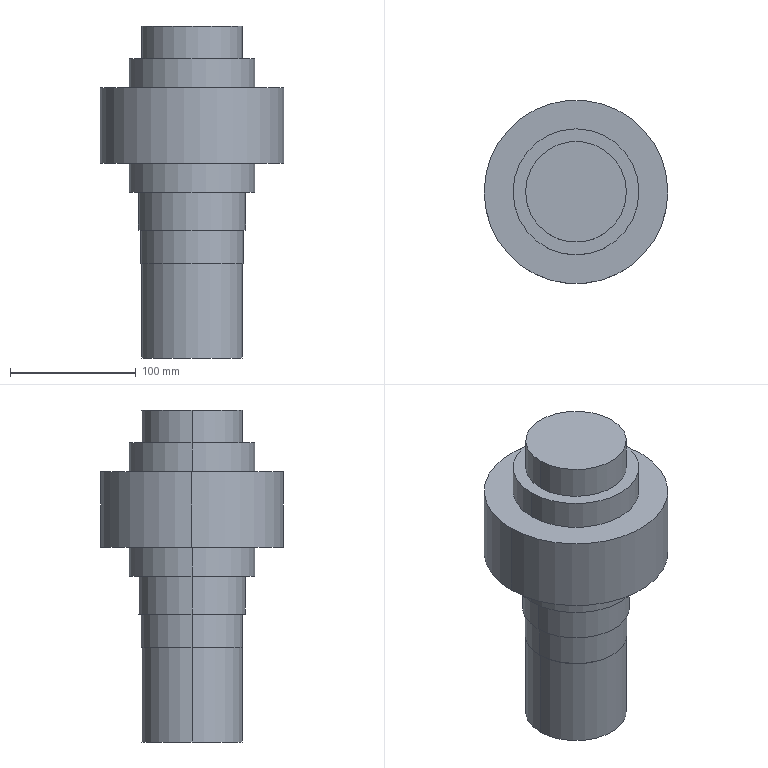Part | SolidWorks | features ICE 6, Extrusion 1 | 1 solid | 22 faces | box 145.723 x 145.723 x 263.5 mm | volume 2176439 mm3 | cylinder 14 | plane 8 | commonest cylinder face diameters 80 x4 100 x4 81 x2 85 x2 145.723 x2
STEP:
#1=CARTESIAN_POINT('',(-40.,0.,-237.5));
#2=VERTEX_POINT('',#1);
#3=CARTESIAN_POINT('',(40.,0.,-237.5));
#4=VERTEX_POINT('',#3);
#5=CARTESIAN_POINT('',(0.,0.,-237.5));
#6=DIRECTION('',(0.,0.,-1.));
#7=DIRECTION('',(-1.,0.,0.));
#8=AXIS2_PLACEMENT_3D('',#5,#6,#7);
#9=CIRCLE('',#8,40.);
#10=EDGE_CURVE('',#2,#4,#9,.T.);
#11=ORIENTED_EDGE('',*,*,#10,.F.);
#12=CARTESIAN_POINT('',(-40.,0.,-162.5));
#13=VERTEX_POINT('',#12);
#14=CARTESIAN_POINT('',(-40.,0.,-237.5));
#15=DIRECTION('',(0.,0.,1.));
#16=VECTOR('',#15,1000.);
#17=LINE('',#14,#16);
#18=EDGE_CURVE('',#2,#13,#17,.T.);
#19=ORIENTED_EDGE('',*,*,#18,.T.);
#20=CARTESIAN_POINT('',(40.,0.,-162.5));
#21=VERTEX_POINT('',#20);
#22=CARTESIAN_POINT('',(0.,0.,-162.5));
#23=DIRECTION('',(0.,0.,-1.));
#24=DIRECTION('',(-1.,0.,0.));
#25=AXIS2_PLACEMENT_3D('',#22,#23,#24);
#26=CIRCLE('',#25,40.);
#27=EDGE_CURVE('',#13,#21,#26,.T.);
#28=ORIENTED_EDGE('',*,*,#27,.T.);
#29=CARTESIAN_POINT('',(40.,0.,-237.5));
#30=DIRECTION('',(0.,0.,1.));
#31=VECTOR('',#30,1000.);
#32=LINE('',#29,#31);
#33=EDGE_CURVE('',#4,#21,#32,.T.);
#34=ORIENTED_EDGE('',*,*,#33,.F.);
#35=EDGE_LOOP('',(#11,#19,#28,#34));
#36=FACE_OUTER_BOUND('',#35,.T.);
#37=CARTESIAN_POINT('',(0.,0.,-237.5));
#38=DIRECTION('',(0.,0.,1.));
#39=DIRECTION('',(1.,0.,0.));
#40=AXIS2_PLACEMENT_3D('',#37,#38,#39);
#41=CYLINDRICAL_SURFACE('',#40,40.);
#42=ADVANCED_FACE('',(#36),#41,.T.);
#43=CARTESIAN_POINT('',(-40.5,0.,-162.5));
#44=VERTEX_POINT('',#43);
#45=CARTESIAN_POINT('',(40.5,0.,-162.5));
#46=VERTEX_POINT('',#45);
#47=CARTESIAN_POINT('',(0.,0.,-162.5));
#48=DIRECTION('',(0.,0.,-1.));
#49=DIRECTION('',(-1.,0.,0.));
#50=AXIS2_PLACEMENT_3D('',#47,#48,#49);
#51=CIRCLE('',#50,40.5);
#52=EDGE_CURVE('',#44,#46,#51,.T.);
#53=ORIENTED_EDGE('',*,*,#52,.F.);
#54=CARTESIAN_POINT('',(-40.5,0.,-136.));
#55=VERTEX_POINT('',#54);
#56=CARTESIAN_POINT('',(-40.5,0.,-162.5));
#57=DIRECTION('',(0.,0.,1.));
#58=VECTOR('',#57,1000.);
#59=LINE('',#56,#58);
#60=EDGE_CURVE('',#44,#55,#59,.T.);
#61=ORIENTED_EDGE('',*,*,#60,.T.);
#62=CARTESIAN_POINT('',(40.5,0.,-136.));
#63=VERTEX_POINT('',#62);
#64=CARTESIAN_POINT('',(0.,0.,-136.));
#65=DIRECTION('',(0.,0.,-1.));
#66=DIRECTION('',(-1.,0.,0.));
#67=AXIS2_PLACEMENT_3D('',#64,#65,#66);
#68=CIRCLE('',#67,40.5);
#69=EDGE_CURVE('',#55,#63,#68,.T.);
#70=ORIENTED_EDGE('',*,*,#69,.T.);
#71=CARTESIAN_POINT('',(40.5,0.,-162.5));
#72=DIRECTION('',(0.,0.,1.));
#73=VECTOR('',#72,1000.);
#74=LINE('',#71,#73);
#75=EDGE_CURVE('',#46,#63,#74,.T.);
#76=ORIENTED_EDGE('',*,*,#75,.F.);
#77=EDGE_LOOP('',(#53,#61,#70,#76));
#78=FACE_OUTER_BOUND('',#77,.T.);
#79=CARTESIAN_POINT('',(0.,0.,-162.5));
#80=DIRECTION('',(0.,0.,1.));
#81=DIRECTION('',(1.,0.,0.));
#82=AXIS2_PLACEMENT_3D('',#79,#80,#81);
#83=CYLINDRICAL_SURFACE('',#82,40.5);
#84=ADVANCED_FACE('',(#78),#83,.T.);
#85=CARTESIAN_POINT('',(-42.5,0.,-136.));
#86=VERTEX_POINT('',#85);
#87=CARTESIAN_POINT('',(42.5,0.,-136.));
#88=VERTEX_POINT('',#87);
#89=CARTESIAN_POINT('',(0.,0.,-136.));
#90=DIRECTION('',(0.,0.,-1.));
#91=DIRECTION('',(-1.,0.,0.));
#92=AXIS2_PLACEMENT_3D('',#89,#90,#91);
#93=CIRCLE('',#92,42.5);
#94=EDGE_CURVE('',#86,#88,#93,.T.);
#95=ORIENTED_EDGE('',*,*,#94,.F.);
#96=CARTESIAN_POINT('',(-42.5,0.,-106.));
#97=VERTEX_POINT('',#96);
#98=CARTESIAN_POINT('',(-42.5,0.,-136.));
#99=DIRECTION('',(0.,0.,1.));
#100=VECTOR('',#99,1000.);
#101=LINE('',#98,#100);
#102=EDGE_CURVE('',#86,#97,#101,.T.);
#103=ORIENTED_EDGE('',*,*,#102,.T.);
#104=CARTESIAN_POINT('',(42.5,0.,-106.));
#105=VERTEX_POINT('',#104);
#106=CARTESIAN_POINT('',(0.,0.,-106.));
#107=DIRECTION('',(0.,0.,-1.));
#108=DIRECTION('',(-1.,0.,0.));
#109=AXIS2_PLACEMENT_3D('',#106,#107,#108);
#110=CIRCLE('',#109,42.5);
#111=EDGE_CURVE('',#97,#105,#110,.T.);
#112=ORIENTED_EDGE('',*,*,#111,.T.);
#113=CARTESIAN_POINT('',(42.5,0.,-136.));
#114=DIRECTION('',(0.,0.,1.));
#115=VECTOR('',#114,1000.);
#116=LINE('',#113,#115);
#117=EDGE_CURVE('',#88,#105,#116,.T.);
#118=ORIENTED_EDGE('',*,*,#117,.F.);
#119=EDGE_LOOP('',(#95,#103,#112,#118));
#120=FACE_OUTER_BOUND('',#119,.T.);
#121=CARTESIAN_POINT('',(0.,0.,-136.));
#122=DIRECTION('',(0.,0.,1.));
#123=DIRECTION('',(1.,0.,0.));
#124=AXIS2_PLACEMENT_3D('',#121,#122,#123);
#125=CYLINDRICAL_SURFACE('',#124,42.5);
#126=ADVANCED_FACE('',(#120),#125,.T.);
#127=CARTESIAN_POINT('',(-50.,0.,-106.));
#128=VERTEX_POINT('',#127);
#129=CARTESIAN_POINT('',(50.,0.,-106.));
#130=VERTEX_POINT('',#129);
#131=CARTESIAN_POINT('',(0.,0.,-106.));
#132=DIRECTION('',(0.,0.,-1.));
#133=DIRECTION('',(-1.,0.,0.));
#134=AXIS2_PLACEMENT_3D('',#131,#132,#133);
#135=CIRCLE('',#134,50.);
#136=EDGE_CURVE('',#128,#130,#135,.T.);
#137=ORIENTED_EDGE('',*,*,#136,.F.);
#138=CARTESIAN_POINT('',(-50.,0.,-83.));
#139=VERTEX_POINT('',#138);
#140=CARTESIAN_POINT('',(-50.,0.,-106.));
#141=DIRECTION('',(0.,0.,1.));
#142=VECTOR('',#141,1000.);
#143=LINE('',#140,#142);
#144=EDGE_CURVE('',#128,#139,#143,.T.);
#145=ORIENTED_EDGE('',*,*,#144,.T.);
#146=CARTESIAN_POINT('',(50.,0.,-83.));
#147=VERTEX_POINT('',#146);
#148=CARTESIAN_POINT('',(0.,0.,-83.));
#149=DIRECTION('',(0.,0.,-1.));
#150=DIRECTION('',(-1.,0.,0.));
#151=AXIS2_PLACEMENT_3D('',#148,#149,#150);
#152=CIRCLE('',#151,50.);
#153=EDGE_CURVE('',#139,#147,#152,.T.);
#154=ORIENTED_EDGE('',*,*,#153,.T.);
#155=CARTESIAN_POINT('',(50.,0.,-106.));
#156=DIRECTION('',(0.,0.,1.));
#157=VECTOR('',#156,1000.);
#158=LINE('',#155,#157);
#159=EDGE_CURVE('',#130,#147,#158,.T.);
#160=ORIENTED_EDGE('',*,*,#159,.F.);
#161=EDGE_LOOP('',(#137,#145,#154,#160));
#162=FACE_OUTER_BOUND('',#161,.T.);
#163=CARTESIAN_POINT('',(0.,0.,-106.));
#164=DIRECTION('',(0.,0.,1.));
#165=DIRECTION('',(1.,0.,0.));
#166=AXIS2_PLACEMENT_3D('',#163,#164,#165);
#167=CYLINDRICAL_SURFACE('',#166,50.);
#168=ADVANCED_FACE('',(#162),#167,.T.);
#169=CARTESIAN_POINT('',(-72.862,0.,-83.));
#170=VERTEX_POINT('',#169);
#171=CARTESIAN_POINT('',(72.862,0.,-83.));
#172=VERTEX_POINT('',#171);
#173=CARTESIAN_POINT('',(0.,0.,-83.));
#174=DIRECTION('',(0.,0.,-1.));
#175=DIRECTION('',(-1.,0.,0.));
#176=AXIS2_PLACEMENT_3D('',#173,#174,#175);
#177=CIRCLE('',#176,72.862);
#178=EDGE_CURVE('',#170,#172,#177,.T.);
#179=ORIENTED_EDGE('',*,*,#178,.F.);
#180=CARTESIAN_POINT('',(-72.862,0.,-23.));
#181=VERTEX_POINT('',#180);
#182=CARTESIAN_POINT('',(-72.862,0.,-83.));
#183=DIRECTION('',(0.,0.,1.));
#184=VECTOR('',#183,1000.);
#185=LINE('',#182,#184);
#186=EDGE_CURVE('',#170,#181,#185,.T.);
#187=ORIENTED_EDGE('',*,*,#186,.T.);
#188=CARTESIAN_POINT('',(72.862,0.,-23.));
#189=VERTEX_POINT('',#188);
#190=CARTESIAN_POINT('',(0.,0.,-23.));
#191=DIRECTION('',(0.,0.,-1.));
#192=DIRECTION('',(-1.,0.,0.));
#193=AXIS2_PLACEMENT_3D('',#190,#191,#192);
#194=CIRCLE('',#193,72.862);
#195=EDGE_CURVE('',#181,#189,#194,.T.);
#196=ORIENTED_EDGE('',*,*,#195,.T.);
#197=CARTESIAN_POINT('',(72.862,0.,-83.));
#198=DIRECTION('',(0.,0.,1.));
#199=VECTOR('',#198,1000.);
#200=LINE('',#197,#199);
#201=EDGE_CURVE('',#172,#189,#200,.T.);
#202=ORIENTED_EDGE('',*,*,#201,.F.);
#203=EDGE_LOOP('',(#179,#187,#196,#202));
#204=FACE_OUTER_BOUND('',#203,.T.);
#205=CARTESIAN_POINT('',(0.,0.,-83.));
#206=DIRECTION('',(0.,0.,1.));
#207=DIRECTION('',(1.,0.,0.));
#208=AXIS2_PLACEMENT_3D('',#205,#206,#207);
#209=CYLINDRICAL_SURFACE('',#208,72.862);
#210=ADVANCED_FACE('',(#204),#209,.T.);
#211=CARTESIAN_POINT('',(-50.,0.,-23.));
#212=VERTEX_POINT('',#211);
#213=CARTESIAN_POINT('',(50.,0.,-23.));
#214=VERTEX_POINT('',#213);
#215=CARTESIAN_POINT('',(0.,0.,-23.));
#216=DIRECTION('',(0.,0.,-1.));
#217=DIRECTION('',(-1.,0.,0.));
#218=AXIS2_PLACEMENT_3D('',#215,#216,#217);
#219=CIRCLE('',#218,50.);
#220=EDGE_CURVE('',#212,#214,#219,.T.);
#221=ORIENTED_EDGE('',*,*,#220,.F.);
#222=CARTESIAN_POINT('',(-50.,0.,0.));
#223=VERTEX_POINT('',#222);
#224=CARTESIAN_POINT('',(-50.,0.,-23.));
#225=DIRECTION('',(0.,0.,1.));
#226=VECTOR('',#225,1000.);
#227=LINE('',#224,#226);
#228=EDGE_CURVE('',#212,#223,#227,.T.);
#229=ORIENTED_EDGE('',*,*,#228,.T.);
#230=CARTESIAN_POINT('',(50.,0.,0.));
#231=VERTEX_POINT('',#230);
#232=CARTESIAN_POINT('',(0.,0.,0.));
#233=DIRECTION('',(0.,0.,-1.));
#234=DIRECTION('',(-1.,0.,0.));
#235=AXIS2_PLACEMENT_3D('',#232,#233,#234);
#236=CIRCLE('',#235,50.);
#237=EDGE_CURVE('',#223,#231,#236,.T.);
#238=ORIENTED_EDGE('',*,*,#237,.T.);
#239=CARTESIAN_POINT('',(50.,0.,-23.));
#240=DIRECTION('',(0.,0.,1.));
#241=VECTOR('',#240,1000.);
#242=LINE('',#239,#241);
#243=EDGE_CURVE('',#214,#231,#242,.T.);
#244=ORIENTED_EDGE('',*,*,#243,.F.);
#245=EDGE_LOOP('',(#221,#229,#238,#244));
#246=FACE_OUTER_BOUND('',#245,.T.);
#247=CARTESIAN_POINT('',(0.,0.,-23.));
#248=DIRECTION('',(0.,0.,1.));
#249=DIRECTION('',(1.,0.,0.));
#250=AXIS2_PLACEMENT_3D('',#247,#248,#249);
#251=CYLINDRICAL_SURFACE('',#250,50.);
#252=ADVANCED_FACE('',(#246),#251,.T.);
#253=CARTESIAN_POINT('',(40.,0.,26.));
#254=VERTEX_POINT('',#253);
#255=CARTESIAN_POINT('',(-40.,0.,26.));
#256=VERTEX_POINT('',#255);
#257=CARTESIAN_POINT('',(0.,0.,26.));
#258=DIRECTION('',(0.,0.,1.));
#259=DIRECTION('',(1.,0.,0.));
#260=AXIS2_PLACEMENT_3D('',#257,#258,#259);
#261=CIRCLE('',#260,40.);
#262=EDGE_CURVE('',#254,#256,#261,.T.);
#263=ORIENTED_EDGE('',*,*,#262,.F.);
#264=CARTESIAN_POINT('',(40.,0.,0.));
#265=VERTEX_POINT('',#264);
#266=CARTESIAN_POINT('',(40.,0.,26.));
#267=DIRECTION('',(0.,0.,-1.));
#268=VECTOR('',#267,1000.);
#269=LINE('',#266,#268);
#270=EDGE_CURVE('',#254,#265,#269,.T.);
#271=ORIENTED_EDGE('',*,*,#270,.T.);
#272=CARTESIAN_POINT('',(-40.,0.,0.));
#273=VERTEX_POINT('',#272);
#274=CARTESIAN_POINT('',(0.,0.,0.));
#275=DIRECTION('',(0.,0.,-1.));
#276=DIRECTION('',(-1.,0.,0.));
#277=AXIS2_PLACEMENT_3D('',#274,#275,#276);
#278=CIRCLE('',#277,40.);
#279=EDGE_CURVE('',#273,#265,#278,.T.);
#280=ORIENTED_EDGE('',*,*,#279,.F.);
#281=CARTESIAN_POINT('',(-40.,0.,26.));
#282=DIRECTION('',(0.,0.,-1.));
#283=VECTOR('',#282,1000.);
#284=LINE('',#281,#283);
#285=EDGE_CURVE('',#256,#273,#284,.T.);
#286=ORIENTED_EDGE('',*,*,#285,.F.);
#287=EDGE_LOOP('',(#263,#271,#280,#286));
#288=FACE_OUTER_BOUND('',#287,.T.);
#289=CARTESIAN_POINT('',(0.,0.,26.));
#290=DIRECTION('',(0.,0.,-1.));
#291=DIRECTION('',(-1.,0.,0.));
#292=AXIS2_PLACEMENT_3D('',#289,#290,#291);
#293=CYLINDRICAL_SURFACE('',#292,40.);
#294=ADVANCED_FACE('',(#288),#293,.T.);
#295=CARTESIAN_POINT('',(0.,0.,-162.5));
#296=DIRECTION('',(0.,0.,-1.));
#297=DIRECTION('',(-1.,0.,0.));
#298=AXIS2_PLACEMENT_3D('',#295,#296,#297);
#299=CIRCLE('',#298,40.5);
#300=EDGE_CURVE('',#46,#44,#299,.T.);
#301=ORIENTED_EDGE('',*,*,#300,.T.);
#302=ORIENTED_EDGE('',*,*,#52,.T.);
#303=EDGE_LOOP('',(#301,#302));
#304=FACE_OUTER_BOUND('',#303,.T.);
#305=CARTESIAN_POINT('',(0.,0.,-162.5));
#306=DIRECTION('',(0.,0.,-1.));
#307=DIRECTION('',(-1.,0.,0.));
#308=AXIS2_PLACEMENT_3D('',#305,#306,#307);
#309=CIRCLE('',#308,40.);
#310=EDGE_CURVE('',#21,#13,#309,.T.);
#311=ORIENTED_EDGE('',*,*,#310,.F.);
#312=ORIENTED_EDGE('',*,*,#27,.F.);
#313=EDGE_LOOP('',(#311,#312));
#314=FACE_BOUND('',#313,.T.);
#315=CARTESIAN_POINT('',(0.,0.,-162.5));
#316=DIRECTION('',(0.,0.,-1.));
#317=DIRECTION('',(-1.,0.,0.));
#318=AXIS2_PLACEMENT_3D('',#315,#316,#317);
#319=PLANE('',#318);
#320=ADVANCED_FACE('',(#304,#314),#319,.T.);
#321=CARTESIAN_POINT('',(0.,0.,-136.));
#322=DIRECTION('',(0.,0.,-1.));
#323=DIRECTION('',(-1.,0.,0.));
#324=AXIS2_PLACEMENT_3D('',#321,#322,#323);
#325=CIRCLE('',#324,42.5);
#326=EDGE_CURVE('',#88,#86,#325,.T.);
#327=ORIENTED_EDGE('',*,*,#326,.T.);
#328=ORIENTED_EDGE('',*,*,#94,.T.);
#329=EDGE_LOOP('',(#327,#328));
#330=FACE_OUTER_BOUND('',#329,.T.);
#331=CARTESIAN_POINT('',(0.,0.,-136.));
#332=DIRECTION('',(0.,0.,-1.));
#333=DIRECTION('',(-1.,0.,0.));
#334=AXIS2_PLACEMENT_3D('',#331,#332,#333);
#335=CIRCLE('',#334,40.5);
#336=EDGE_CURVE('',#63,#55,#335,.T.);
#337=ORIENTED_EDGE('',*,*,#336,.F.);
#338=ORIENTED_EDGE('',*,*,#69,.F.);
#339=EDGE_LOOP('',(#337,#338));
#340=FACE_BOUND('',#339,.T.);
#341=CARTESIAN_POINT('',(0.,0.,-136.));
#342=DIRECTION('',(0.,0.,-1.));
#343=DIRECTION('',(-1.,0.,0.));
#344=AXIS2_PLACEMENT_3D('',#341,#342,#343);
#345=PLANE('',#344);
#346=ADVANCED_FACE('',(#330,#340),#345,.T.);
#347=CARTESIAN_POINT('',(0.,0.,-106.));
#348=DIRECTION('',(0.,0.,-1.));
#349=DIRECTION('',(-1.,0.,0.));
#350=AXIS2_PLACEMENT_3D('',#347,#348,#349);
#351=CIRCLE('',#350,50.);
#352=EDGE_CURVE('',#130,#128,#351,.T.);
#353=ORIENTED_EDGE('',*,*,#352,.T.);
#354=ORIENTED_EDGE('',*,*,#136,.T.);
#355=EDGE_LOOP('',(#353,#354));
#356=FACE_OUTER_BOUND('',#355,.T.);
#357=CARTESIAN_POINT('',(0.,0.,-106.));
#358=DIRECTION('',(0.,0.,-1.));
#359=DIRECTION('',(-1.,0.,0.));
#360=AXIS2_PLACEMENT_3D('',#357,#358,#359);
#361=CIRCLE('',#360,42.5);
#362=EDGE_CURVE('',#105,#97,#361,.T.);
#363=ORIENTED_EDGE('',*,*,#362,.F.);
#364=ORIENTED_EDGE('',*,*,#111,.F.);
#365=EDGE_LOOP('',(#363,#364));
#366=FACE_BOUND('',#365,.T.);
#367=CARTESIAN_POINT('',(0.,0.,-106.));
#368=DIRECTION('',(0.,0.,-1.));
#369=DIRECTION('',(-1.,0.,0.));
#370=AXIS2_PLACEMENT_3D('',#367,#368,#369);
#371=PLANE('',#370);
#372=ADVANCED_FACE('',(#356,#366),#371,.T.);
#373=CARTESIAN_POINT('',(0.,0.,-83.));
#374=DIRECTION('',(0.,0.,-1.));
#375=DIRECTION('',(-1.,0.,0.));
#376=AXIS2_PLACEMENT_3D('',#373,#374,#375);
#377=CIRCLE('',#376,72.862);
#378=EDGE_CURVE('',#172,#170,#377,.T.);
#379=ORIENTED_EDGE('',*,*,#378,.T.);
#380=ORIENTED_EDGE('',*,*,#178,.T.);
#381=EDGE_LOOP('',(#379,#380));
#382=FACE_OUTER_BOUND('',#381,.T.);
#383=CARTESIAN_POINT('',(0.,0.,-83.));
#384=DIRECTION('',(0.,0.,-1.));
#385=DIRECTION('',(-1.,0.,0.));
#386=AXIS2_PLACEMENT_3D('',#383,#384,#385);
#387=CIRCLE('',#386,50.);
#388=EDGE_CURVE('',#147,#139,#387,.T.);
#389=ORIENTED_EDGE('',*,*,#388,.F.);
#390=ORIENTED_EDGE('',*,*,#153,.F.);
#391=EDGE_LOOP('',(#389,#390));
#392=FACE_BOUND('',#391,.T.);
#393=CARTESIAN_POINT('',(0.,0.,-83.));
#394=DIRECTION('',(0.,0.,-1.));
#395=DIRECTION('',(-1.,0.,0.));
#396=AXIS2_PLACEMENT_3D('',#393,#394,#395);
#397=PLANE('',#396);
#398=ADVANCED_FACE('',(#382,#392),#397,.T.);
#399=ORIENTED_EDGE('',*,*,#270,.F.);
#400=CARTESIAN_POINT('',(0.,0.,26.));
#401=DIRECTION('',(0.,0.,1.));
#402=DIRECTION('',(1.,0.,0.));
#403=AXIS2_PLACEMENT_3D('',#400,#401,#402);
#404=CIRCLE('',#403,40.);
#405=EDGE_CURVE('',#256,#254,#404,.T.);
#406=ORIENTED_EDGE('',*,*,#405,.F.);
#407=ORIENTED_EDGE('',*,*,#285,.T.);
#408=CARTESIAN_POINT('',(0.,0.,0.));
#409=DIRECTION('',(0.,0.,-1.));
#410=DIRECTION('',(-1.,0.,0.));
#411=AXIS2_PLACEMENT_3D('',#408,#409,#410);
#412=CIRCLE('',#411,40.);
#413=EDGE_CURVE('',#265,#273,#412,.T.);
#414=ORIENTED_EDGE('',*,*,#413,.F.);
#415=EDGE_LOOP('',(#399,#406,#407,#414));
#416=FACE_OUTER_BOUND('',#415,.T.);
#417=CARTESIAN_POINT('',(0.,0.,26.));
#418=DIRECTION('',(0.,0.,-1.));
#419=DIRECTION('',(-1.,0.,0.));
#420=AXIS2_PLACEMENT_3D('',#417,#418,#419);
#421=CYLINDRICAL_SURFACE('',#420,40.);
#422=ADVANCED_FACE('',(#416),#421,.T.);
#423=ORIENTED_EDGE('',*,*,#405,.T.);
#424=ORIENTED_EDGE('',*,*,#262,.T.);
#425=EDGE_LOOP('',(#423,#424));
#426=FACE_OUTER_BOUND('',#425,.T.);
#427=CARTESIAN_POINT('',(0.,0.,26.));
#428=DIRECTION('',(0.,0.,1.));
#429=DIRECTION('',(1.,0.,0.));
#430=AXIS2_PLACEMENT_3D('',#427,#428,#429);
#431=PLANE('',#430);
#432=ADVANCED_FACE('',(#426),#431,.T.);
#433=CARTESIAN_POINT('',(0.,0.,0.));
#434=DIRECTION('',(0.,0.,-1.));
#435=DIRECTION('',(-1.,0.,0.));
#436=AXIS2_PLACEMENT_3D('',#433,#434,#435);
#437=CIRCLE('',#436,50.);
#438=EDGE_CURVE('',#231,#223,#437,.T.);
#439=ORIENTED_EDGE('',*,*,#438,.F.);
#440=ORIENTED_EDGE('',*,*,#237,.F.);
#441=EDGE_LOOP('',(#439,#440));
#442=FACE_OUTER_BOUND('',#441,.T.);
#443=ORIENTED_EDGE('',*,*,#279,.T.);
#444=ORIENTED_EDGE('',*,*,#413,.T.);
#445=EDGE_LOOP('',(#443,#444));
#446=FACE_BOUND('',#445,.T.);
#447=CARTESIAN_POINT('',(0.,0.,0.));
#448=DIRECTION('',(0.,0.,-1.));
#449=DIRECTION('',(-1.,0.,0.));
#450=AXIS2_PLACEMENT_3D('',#447,#448,#449);
#451=PLANE('',#450);
#452=ADVANCED_FACE('',(#442,#446),#451,.F.);
#453=ORIENTED_EDGE('',*,*,#228,.F.);
#454=CARTESIAN_POINT('',(0.,0.,-23.));
#455=DIRECTION('',(0.,0.,-1.));
#456=DIRECTION('',(-1.,0.,0.));
#457=AXIS2_PLACEMENT_3D('',#454,#455,#456);
#458=CIRCLE('',#457,50.);
#459=EDGE_CURVE('',#214,#212,#458,.T.);
#460=ORIENTED_EDGE('',*,*,#459,.F.);
#461=ORIENTED_EDGE('',*,*,#243,.T.);
#462=ORIENTED_EDGE('',*,*,#438,.T.);
#463=EDGE_LOOP('',(#453,#460,#461,#462));
#464=FACE_OUTER_BOUND('',#463,.T.);
#465=CARTESIAN_POINT('',(0.,0.,-23.));
#466=DIRECTION('',(0.,0.,1.));
#467=DIRECTION('',(1.,0.,0.));
#468=AXIS2_PLACEMENT_3D('',#465,#466,#467);
#469=CYLINDRICAL_SURFACE('',#468,50.);
#470=ADVANCED_FACE('',(#464),#469,.T.);
#471=CARTESIAN_POINT('',(0.,0.,-23.));
#472=DIRECTION('',(0.,0.,-1.));
#473=DIRECTION('',(-1.,0.,0.));
#474=AXIS2_PLACEMENT_3D('',#471,#472,#473);
#475=CIRCLE('',#474,72.862);
#476=EDGE_CURVE('',#189,#181,#475,.T.);
#477=ORIENTED_EDGE('',*,*,#476,.F.);
#478=ORIENTED_EDGE('',*,*,#195,.F.);
#479=EDGE_LOOP('',(#477,#478));
#480=FACE_OUTER_BOUND('',#479,.T.);
#481=ORIENTED_EDGE('',*,*,#459,.T.);
#482=ORIENTED_EDGE('',*,*,#220,.T.);
#483=EDGE_LOOP('',(#481,#482));
#484=FACE_BOUND('',#483,.T.);
#485=CARTESIAN_POINT('',(0.,0.,-23.));
#486=DIRECTION('',(0.,0.,-1.));
#487=DIRECTION('',(-1.,0.,0.));
#488=AXIS2_PLACEMENT_3D('',#485,#486,#487);
#489=PLANE('',#488);
#490=ADVANCED_FACE('',(#480,#484),#489,.F.);
#491=ORIENTED_EDGE('',*,*,#186,.F.);
#492=ORIENTED_EDGE('',*,*,#378,.F.);
#493=ORIENTED_EDGE('',*,*,#201,.T.);
#494=ORIENTED_EDGE('',*,*,#476,.T.);
#495=EDGE_LOOP('',(#491,#492,#493,#494));
#496=FACE_OUTER_BOUND('',#495,.T.);
#497=CARTESIAN_POINT('',(0.,0.,-83.));
#498=DIRECTION('',(0.,0.,1.));
#499=DIRECTION('',(1.,0.,0.));
#500=AXIS2_PLACEMENT_3D('',#497,#498,#499);
#501=CYLINDRICAL_SURFACE('',#500,72.862);
#502=ADVANCED_FACE('',(#496),#501,.T.);
#503=ORIENTED_EDGE('',*,*,#144,.F.);
#504=ORIENTED_EDGE('',*,*,#352,.F.);
#505=ORIENTED_EDGE('',*,*,#159,.T.);
#506=ORIENTED_EDGE('',*,*,#388,.T.);
#507=EDGE_LOOP('',(#503,#504,#505,#506));
#508=FACE_OUTER_BOUND('',#507,.T.);
#509=CARTESIAN_POINT('',(0.,0.,-106.));
#510=DIRECTION('',(0.,0.,1.));
#511=DIRECTION('',(1.,0.,0.));
#512=AXIS2_PLACEMENT_3D('',#509,#510,#511);
#513=CYLINDRICAL_SURFACE('',#512,50.);
#514=ADVANCED_FACE('',(#508),#513,.T.);
#515=ORIENTED_EDGE('',*,*,#102,.F.);
#516=ORIENTED_EDGE('',*,*,#326,.F.);
#517=ORIENTED_EDGE('',*,*,#117,.T.);
#518=ORIENTED_EDGE('',*,*,#362,.T.);
#519=EDGE_LOOP('',(#515,#516,#517,#518));
#520=FACE_OUTER_BOUND('',#519,.T.);
#521=CARTESIAN_POINT('',(0.,0.,-136.));
#522=DIRECTION('',(0.,0.,1.));
#523=DIRECTION('',(1.,0.,0.));
#524=AXIS2_PLACEMENT_3D('',#521,#522,#523);
#525=CYLINDRICAL_SURFACE('',#524,42.5);
#526=ADVANCED_FACE('',(#520),#525,.T.);
#527=ORIENTED_EDGE('',*,*,#60,.F.);
#528=ORIENTED_EDGE('',*,*,#300,.F.);
#529=ORIENTED_EDGE('',*,*,#75,.T.);
#530=ORIENTED_EDGE('',*,*,#336,.T.);
#531=EDGE_LOOP('',(#527,#528,#529,#530));
#532=FACE_OUTER_BOUND('',#531,.T.);
#533=CARTESIAN_POINT('',(0.,0.,-162.5));
#534=DIRECTION('',(0.,0.,1.));
#535=DIRECTION('',(1.,0.,0.));
#536=AXIS2_PLACEMENT_3D('',#533,#534,#535);
#537=CYLINDRICAL_SURFACE('',#536,40.5);
#538=ADVANCED_FACE('',(#532),#537,.T.);
#539=ORIENTED_EDGE('',*,*,#18,.F.);
#540=CARTESIAN_POINT('',(0.,0.,-237.5));
#541=DIRECTION('',(0.,0.,-1.));
#542=DIRECTION('',(-1.,0.,0.));
#543=AXIS2_PLACEMENT_3D('',#540,#541,#542);
#544=CIRCLE('',#543,40.);
#545=EDGE_CURVE('',#4,#2,#544,.T.);
#546=ORIENTED_EDGE('',*,*,#545,.F.);
#547=ORIENTED_EDGE('',*,*,#33,.T.);
#548=ORIENTED_EDGE('',*,*,#310,.T.);
#549=EDGE_LOOP('',(#539,#546,#547,#548));
#550=FACE_OUTER_BOUND('',#549,.T.);
#551=CARTESIAN_POINT('',(0.,0.,-237.5));
#552=DIRECTION('',(0.,0.,1.));
#553=DIRECTION('',(1.,0.,0.));
#554=AXIS2_PLACEMENT_3D('',#551,#552,#553);
#555=CYLINDRICAL_SURFACE('',#554,40.);
#556=ADVANCED_FACE('',(#550),#555,.T.);
#557=ORIENTED_EDGE('',*,*,#545,.T.);
#558=ORIENTED_EDGE('',*,*,#10,.T.);
#559=EDGE_LOOP('',(#557,#558));
#560=FACE_OUTER_BOUND('',#559,.T.);
#561=CARTESIAN_POINT('',(0.,0.,-237.5));
#562=DIRECTION('',(0.,0.,-1.));
#563=DIRECTION('',(-1.,0.,0.));
#564=AXIS2_PLACEMENT_3D('',#561,#562,#563);
#565=PLANE('',#564);
#566=ADVANCED_FACE('',(#560),#565,.T.);
#567=CLOSED_SHELL('',(#42,#84,#126,#168,#210,#252,#294,#320,#346,#372,#398,#422,#432,#452,#470,#490,#502,#514,#526,#538,#556,#566));
#568=MANIFOLD_SOLID_BREP('',#567);
#569=CARTESIAN_POINT('',(0.,0.,0.));
#570=DIRECTION('',(0.,0.,1.));
#571=DIRECTION('',(1.,0.,0.));
#572=AXIS2_PLACEMENT_3D('',#569,#570,#571);
#573=(LENGTH_UNIT()NAMED_UNIT(*)SI_UNIT(.MILLI.,.METRE.));
#574=UNCERTAINTY_MEASURE_WITH_UNIT(LENGTH_MEASURE(0.00001),#573,'','');
#575=(NAMED_UNIT(*)PLANE_ANGLE_UNIT()SI_UNIT($,.RADIAN.));
#576=(NAMED_UNIT(*)SI_UNIT($,.STERADIAN.)SOLID_ANGLE_UNIT());
#577=(GEOMETRIC_REPRESENTATION_CONTEXT(3)GLOBAL_UNCERTAINTY_ASSIGNED_CONTEXT((#574))GLOBAL_UNIT_ASSIGNED_CONTEXT((#573,#575,#576))REPRESENTATION_CONTEXT('',''));
#578=ADVANCED_BREP_SHAPE_REPRESENTATION('',(#568,#572),#577);